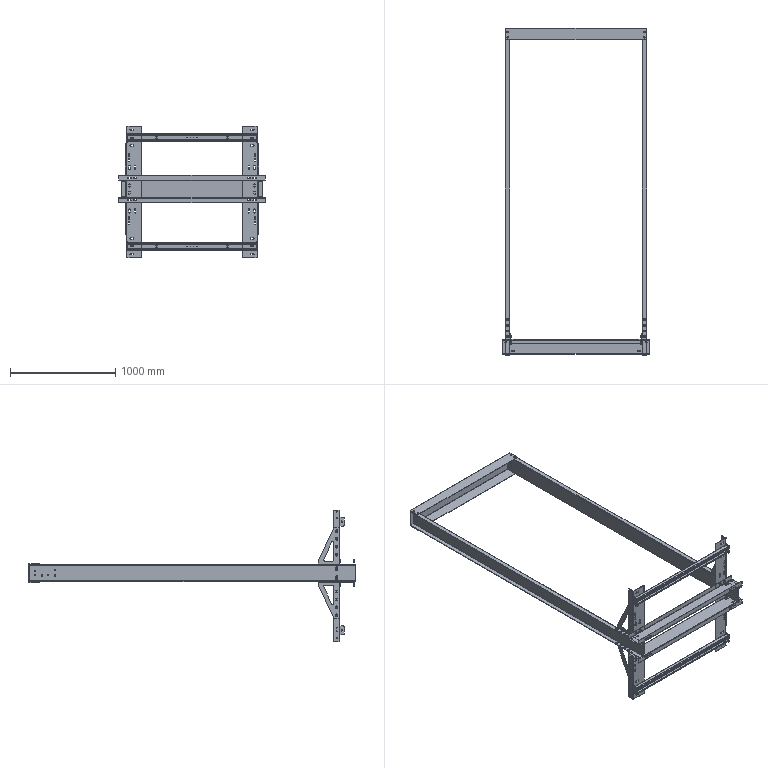Part | 45 solids | 1824 faces | box 1390 x 3110 x 1255 mm | volume 17049854 mm3 | plane 956 | cylinder 700 | cone 168 | commonest cylinder face diameters 13 x180 14 x156 10.647 x56 14.75 x56 15.07 x56 15 x40